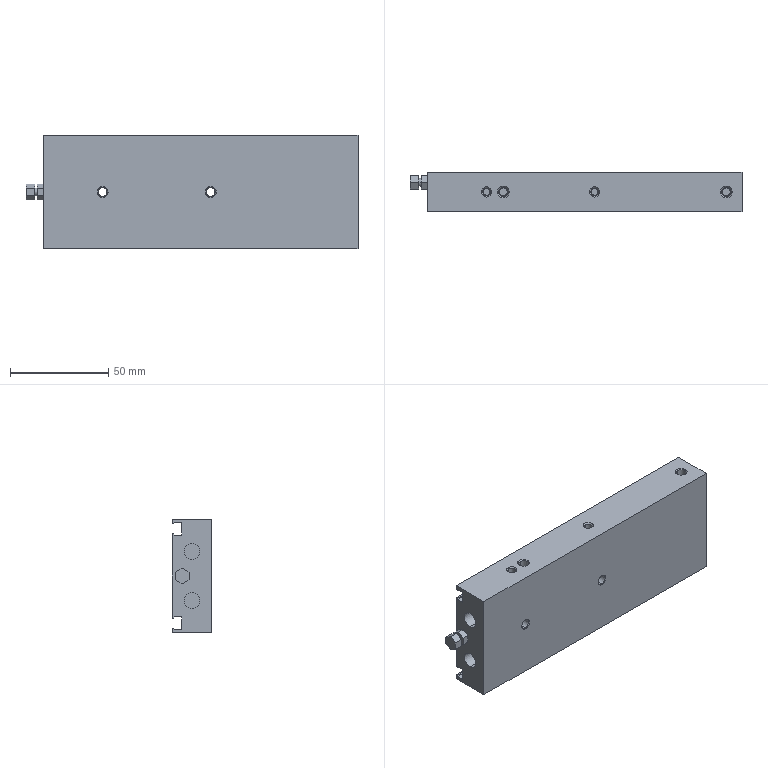Part | NX | 1 solid | 163 faces | box 169 x 20 x 58 mm | volume 157802 mm3 | cylinder 62 | plane 53 | cone 48 | commonest cylinder face diameters 4 x18 5 x12 3.4 x8 4.5 x8 8 x8 4.3 x4